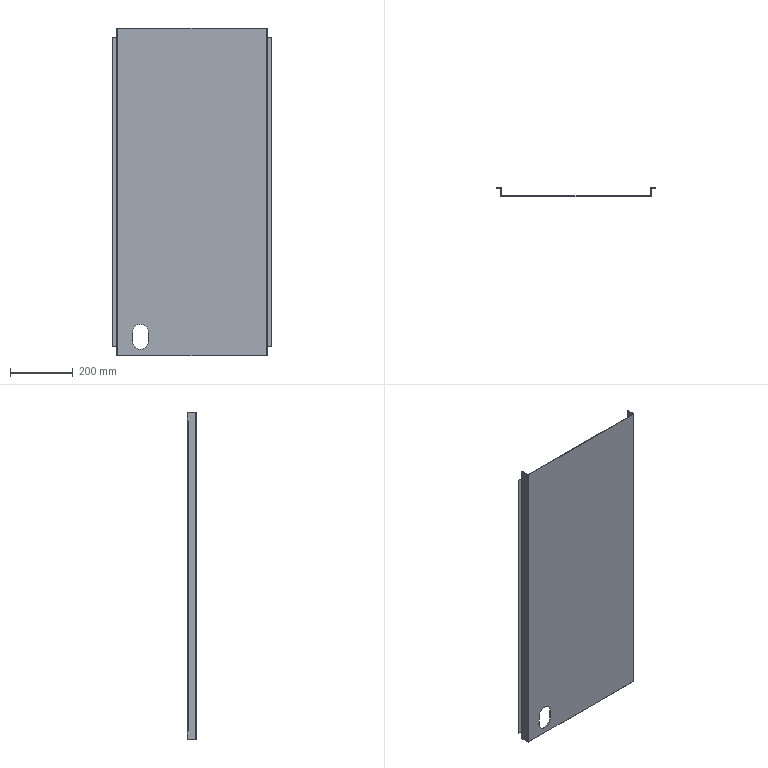Part | SolidWorks | features EdgeFlange 2, FlatPattern 1, ICE 1, SMBaseFlange 1, SheetMetal 1 | 1 solid | 51 faces | box 510 x 30 x 1047 mm | volume 876812 mm3 | plane 40 | cylinder 11 | commonest cylinder face diameters 3 x4 6 x4 50 x3
STEP:
#1=CARTESIAN_POINT('',(63.279,-16.571,45.));
#2=VERTEX_POINT('',#1);
#3=CARTESIAN_POINT('',(38.279,-16.571,20.));
#4=VERTEX_POINT('',#3);
#5=CARTESIAN_POINT('',(38.279,-16.571,45.));
#6=DIRECTION('',(0.,1.,0.));
#7=DIRECTION('',(0.,0.,1.));
#8=AXIS2_PLACEMENT_3D('',#5,#6,#7);
#9=CIRCLE('',#8,25.);
#10=EDGE_CURVE('',#2,#4,#9,.T.);
#11=ORIENTED_EDGE('',*,*,#10,.T.);
#12=CARTESIAN_POINT('',(38.279,-18.071,20.));
#13=VERTEX_POINT('',#12);
#14=CARTESIAN_POINT('',(38.279,-8.071,20.));
#15=DIRECTION('',(0.,-1.,0.));
#16=VECTOR('',#15,1000.);
#17=LINE('',#14,#16);
#18=EDGE_CURVE('',#4,#13,#17,.T.);
#19=ORIENTED_EDGE('',*,*,#18,.T.);
#20=CARTESIAN_POINT('',(63.279,-18.071,45.));
#21=VERTEX_POINT('',#20);
#22=CARTESIAN_POINT('',(38.279,-18.071,45.));
#23=DIRECTION('',(0.,-1.,0.));
#24=DIRECTION('',(0.,0.,-1.));
#25=AXIS2_PLACEMENT_3D('',#22,#23,#24);
#26=CIRCLE('',#25,25.);
#27=EDGE_CURVE('',#13,#21,#26,.T.);
#28=ORIENTED_EDGE('',*,*,#27,.T.);
#29=CARTESIAN_POINT('',(63.279,-8.071,45.));
#30=DIRECTION('',(0.,-1.,0.));
#31=VECTOR('',#30,1000.);
#32=LINE('',#29,#31);
#33=EDGE_CURVE('',#2,#21,#32,.T.);
#34=ORIENTED_EDGE('',*,*,#33,.F.);
#35=EDGE_LOOP('',(#11,#19,#28,#34));
#36=FACE_OUTER_BOUND('',#35,.T.);
#37=CARTESIAN_POINT('',(38.279,-8.071,45.));
#38=DIRECTION('',(0.,-1.,0.));
#39=DIRECTION('',(0.,0.,-1.));
#40=AXIS2_PLACEMENT_3D('',#37,#38,#39);
#41=CYLINDRICAL_SURFACE('',#40,25.);
#42=ADVANCED_FACE('',(#36),#41,.F.);
#43=CARTESIAN_POINT('',(-36.721,11.929,28.5));
#44=VERTEX_POINT('',#43);
#45=CARTESIAN_POINT('',(-36.721,11.527,28.5));
#46=VERTEX_POINT('',#45);
#47=CARTESIAN_POINT('',(-36.721,11.929,28.5));
#48=DIRECTION('',(0.,-1.,0.));
#49=VECTOR('',#48,1000.);
#50=LINE('',#47,#49);
#51=EDGE_CURVE('',#44,#46,#50,.T.);
#52=ORIENTED_EDGE('',*,*,#51,.T.);
#53=CARTESIAN_POINT('',(-35.221,8.929,28.5));
#54=VERTEX_POINT('',#53);
#55=CARTESIAN_POINT('',(-38.221,8.929,28.5));
#56=DIRECTION('',(0.,0.,-1.));
#57=DIRECTION('',(-1.,0.,0.));
#58=AXIS2_PLACEMENT_3D('',#55,#56,#57);
#59=CIRCLE('',#58,3.);
#60=EDGE_CURVE('',#46,#54,#59,.T.);
#61=ORIENTED_EDGE('',*,*,#60,.T.);
#62=CARTESIAN_POINT('',(-35.221,11.929,28.5));
#63=VERTEX_POINT('',#62);
#64=CARTESIAN_POINT('',(-35.221,0.,28.5));
#65=DIRECTION('',(0.,-1.,0.));
#66=VECTOR('',#65,1000.);
#67=LINE('',#64,#66);
#68=EDGE_CURVE('',#63,#54,#67,.T.);
#69=ORIENTED_EDGE('',*,*,#68,.F.);
#70=CARTESIAN_POINT('',(-36.721,11.929,28.5));
#71=DIRECTION('',(1.,0.,0.));
#72=VECTOR('',#71,1000.);
#73=LINE('',#70,#72);
#74=EDGE_CURVE('',#44,#63,#73,.T.);
#75=ORIENTED_EDGE('',*,*,#74,.F.);
#76=EDGE_LOOP('',(#52,#61,#69,#75));
#77=FACE_OUTER_BOUND('',#76,.T.);
#78=CARTESIAN_POINT('',(-36.721,11.929,28.5));
#79=DIRECTION('',(0.,0.,1.));
#80=DIRECTION('',(0.,-1.,0.));
#81=AXIS2_PLACEMENT_3D('',#78,#79,#80);
#82=PLANE('',#81);
#83=ADVANCED_FACE('',(#77),#82,.T.);
#84=CARTESIAN_POINT('',(-35.221,8.929,1018.5));
#85=VERTEX_POINT('',#84);
#86=CARTESIAN_POINT('',(-35.221,11.929,1018.5));
#87=VERTEX_POINT('',#86);
#88=CARTESIAN_POINT('',(-35.221,0.,1018.5));
#89=DIRECTION('',(0.,1.,0.));
#90=VECTOR('',#89,1000.);
#91=LINE('',#88,#90);
#92=EDGE_CURVE('',#85,#87,#91,.T.);
#93=ORIENTED_EDGE('',*,*,#92,.F.);
#94=CARTESIAN_POINT('',(-36.721,11.527,1018.5));
#95=VERTEX_POINT('',#94);
#96=CARTESIAN_POINT('',(-38.221,8.929,1018.5));
#97=DIRECTION('',(0.,0.,1.));
#98=DIRECTION('',(-1.,0.,0.));
#99=AXIS2_PLACEMENT_3D('',#96,#97,#98);
#100=CIRCLE('',#99,3.);
#101=EDGE_CURVE('',#85,#95,#100,.T.);
#102=ORIENTED_EDGE('',*,*,#101,.T.);
#103=CARTESIAN_POINT('',(-36.721,11.929,1018.5));
#104=VERTEX_POINT('',#103);
#105=CARTESIAN_POINT('',(-36.721,8.929,1018.5));
#106=DIRECTION('',(0.,1.,0.));
#107=VECTOR('',#106,1000.);
#108=LINE('',#105,#107);
#109=EDGE_CURVE('',#95,#104,#108,.T.);
#110=ORIENTED_EDGE('',*,*,#109,.T.);
#111=CARTESIAN_POINT('',(-36.721,11.929,1018.5));
#112=DIRECTION('',(1.,0.,0.));
#113=VECTOR('',#112,1000.);
#114=LINE('',#111,#113);
#115=EDGE_CURVE('',#104,#87,#114,.T.);
#116=ORIENTED_EDGE('',*,*,#115,.T.);
#117=EDGE_LOOP('',(#93,#102,#110,#116));
#118=FACE_OUTER_BOUND('',#117,.T.);
#119=CARTESIAN_POINT('',(-36.721,8.929,1018.5));
#120=DIRECTION('',(0.,0.,-1.));
#121=DIRECTION('',(-1.,0.,0.));
#122=AXIS2_PLACEMENT_3D('',#119,#120,#121);
#123=PLANE('',#122);
#124=ADVANCED_FACE('',(#118),#123,.T.);
#125=CARTESIAN_POINT('',(443.279,11.929,1018.5));
#126=VERTEX_POINT('',#125);
#127=CARTESIAN_POINT('',(443.279,11.527,1018.5));
#128=VERTEX_POINT('',#127);
#129=CARTESIAN_POINT('',(443.279,11.929,1018.5));
#130=DIRECTION('',(0.,-1.,0.));
#131=VECTOR('',#130,1000.);
#132=LINE('',#129,#131);
#133=EDGE_CURVE('',#126,#128,#132,.T.);
#134=ORIENTED_EDGE('',*,*,#133,.T.);
#135=CARTESIAN_POINT('',(441.779,8.929,1018.5));
#136=VERTEX_POINT('',#135);
#137=CARTESIAN_POINT('',(444.779,8.929,1018.5));
#138=DIRECTION('',(0.,0.,1.));
#139=DIRECTION('',(1.,0.,0.));
#140=AXIS2_PLACEMENT_3D('',#137,#138,#139);
#141=CIRCLE('',#140,3.);
#142=EDGE_CURVE('',#128,#136,#141,.T.);
#143=ORIENTED_EDGE('',*,*,#142,.T.);
#144=CARTESIAN_POINT('',(441.779,11.929,1018.5));
#145=VERTEX_POINT('',#144);
#146=CARTESIAN_POINT('',(441.779,0.,1018.5));
#147=DIRECTION('',(0.,1.,0.));
#148=VECTOR('',#147,1000.);
#149=LINE('',#146,#148);
#150=EDGE_CURVE('',#136,#145,#149,.T.);
#151=ORIENTED_EDGE('',*,*,#150,.T.);
#152=CARTESIAN_POINT('',(443.279,11.929,1018.5));
#153=DIRECTION('',(-1.,0.,0.));
#154=VECTOR('',#153,1000.);
#155=LINE('',#152,#154);
#156=EDGE_CURVE('',#126,#145,#155,.T.);
#157=ORIENTED_EDGE('',*,*,#156,.F.);
#158=EDGE_LOOP('',(#134,#143,#151,#157));
#159=FACE_OUTER_BOUND('',#158,.T.);
#160=CARTESIAN_POINT('',(443.279,11.929,1018.5));
#161=DIRECTION('',(0.,0.,-1.));
#162=DIRECTION('',(-1.,0.,0.));
#163=AXIS2_PLACEMENT_3D('',#160,#161,#162);
#164=PLANE('',#163);
#165=ADVANCED_FACE('',(#159),#164,.T.);
#166=CARTESIAN_POINT('',(441.779,11.929,28.5));
#167=VERTEX_POINT('',#166);
#168=CARTESIAN_POINT('',(441.779,8.929,28.5));
#169=VERTEX_POINT('',#168);
#170=CARTESIAN_POINT('',(441.779,0.,28.5));
#171=DIRECTION('',(0.,-1.,0.));
#172=VECTOR('',#171,1000.);
#173=LINE('',#170,#172);
#174=EDGE_CURVE('',#167,#169,#173,.T.);
#175=ORIENTED_EDGE('',*,*,#174,.T.);
#176=CARTESIAN_POINT('',(443.279,11.527,28.5));
#177=VERTEX_POINT('',#176);
#178=CARTESIAN_POINT('',(444.779,8.929,28.5));
#179=DIRECTION('',(0.,0.,-1.));
#180=DIRECTION('',(1.,0.,0.));
#181=AXIS2_PLACEMENT_3D('',#178,#179,#180);
#182=CIRCLE('',#181,3.);
#183=EDGE_CURVE('',#169,#177,#182,.T.);
#184=ORIENTED_EDGE('',*,*,#183,.T.);
#185=CARTESIAN_POINT('',(443.279,11.929,28.5));
#186=VERTEX_POINT('',#185);
#187=CARTESIAN_POINT('',(443.279,8.929,28.5));
#188=DIRECTION('',(0.,1.,0.));
#189=VECTOR('',#188,1000.);
#190=LINE('',#187,#189);
#191=EDGE_CURVE('',#177,#186,#190,.T.);
#192=ORIENTED_EDGE('',*,*,#191,.T.);
#193=CARTESIAN_POINT('',(443.279,11.929,28.5));
#194=DIRECTION('',(-1.,0.,0.));
#195=VECTOR('',#194,1000.);
#196=LINE('',#193,#195);
#197=EDGE_CURVE('',#186,#167,#196,.T.);
#198=ORIENTED_EDGE('',*,*,#197,.T.);
#199=EDGE_LOOP('',(#175,#184,#192,#198));
#200=FACE_OUTER_BOUND('',#199,.T.);
#201=CARTESIAN_POINT('',(443.279,8.929,28.5));
#202=DIRECTION('',(0.,0.,1.));
#203=DIRECTION('',(1.,0.,0.));
#204=AXIS2_PLACEMENT_3D('',#201,#202,#203);
#205=PLANE('',#204);
#206=ADVANCED_FACE('',(#200),#205,.T.);
#207=ORIENTED_EDGE('',*,*,#51,.F.);
#208=CARTESIAN_POINT('',(-36.721,11.929,0.));
#209=VERTEX_POINT('',#208);
#210=CARTESIAN_POINT('',(-36.721,11.929,0.));
#211=DIRECTION('',(0.,0.,1.));
#212=VECTOR('',#211,1000.);
#213=LINE('',#210,#212);
#214=EDGE_CURVE('',#209,#44,#213,.T.);
#215=ORIENTED_EDGE('',*,*,#214,.F.);
#216=CARTESIAN_POINT('',(-36.721,-15.071,0.));
#217=VERTEX_POINT('',#216);
#218=CARTESIAN_POINT('',(-36.721,-16.571,0.));
#219=DIRECTION('',(0.,1.,0.));
#220=VECTOR('',#219,1000.);
#221=LINE('',#218,#220);
#222=EDGE_CURVE('',#217,#209,#221,.T.);
#223=ORIENTED_EDGE('',*,*,#222,.F.);
#224=CARTESIAN_POINT('',(-36.721,-15.071,1047.));
#225=VERTEX_POINT('',#224);
#226=CARTESIAN_POINT('',(-36.721,-15.071,0.));
#227=DIRECTION('',(0.,0.,-1.));
#228=VECTOR('',#227,1000.);
#229=LINE('',#226,#228);
#230=EDGE_CURVE('',#225,#217,#229,.T.);
#231=ORIENTED_EDGE('',*,*,#230,.F.);
#232=CARTESIAN_POINT('',(-36.721,11.929,1047.));
#233=VERTEX_POINT('',#232);
#234=CARTESIAN_POINT('',(-36.721,11.929,1047.));
#235=DIRECTION('',(0.,-1.,0.));
#236=VECTOR('',#235,1000.);
#237=LINE('',#234,#236);
#238=EDGE_CURVE('',#233,#225,#237,.T.);
#239=ORIENTED_EDGE('',*,*,#238,.F.);
#240=CARTESIAN_POINT('',(-36.721,11.929,0.));
#241=DIRECTION('',(0.,0.,1.));
#242=VECTOR('',#241,1000.);
#243=LINE('',#240,#242);
#244=EDGE_CURVE('',#104,#233,#243,.T.);
#245=ORIENTED_EDGE('',*,*,#244,.F.);
#246=ORIENTED_EDGE('',*,*,#109,.F.);
#247=CARTESIAN_POINT('',(-36.721,8.929,1018.5));
#248=VERTEX_POINT('',#247);
#249=CARTESIAN_POINT('',(-36.721,8.929,1018.5));
#250=DIRECTION('',(0.,1.,0.));
#251=VECTOR('',#250,1000.);
#252=LINE('',#249,#251);
#253=EDGE_CURVE('',#248,#95,#252,.T.);
#254=ORIENTED_EDGE('',*,*,#253,.F.);
#255=CARTESIAN_POINT('',(-36.721,8.929,28.5));
#256=VERTEX_POINT('',#255);
#257=CARTESIAN_POINT('',(-36.721,8.929,28.5));
#258=DIRECTION('',(0.,0.,1.));
#259=VECTOR('',#258,1000.);
#260=LINE('',#257,#259);
#261=EDGE_CURVE('',#256,#248,#260,.T.);
#262=ORIENTED_EDGE('',*,*,#261,.F.);
#263=CARTESIAN_POINT('',(-36.721,11.929,28.5));
#264=DIRECTION('',(0.,-1.,0.));
#265=VECTOR('',#264,1000.);
#266=LINE('',#263,#265);
#267=EDGE_CURVE('',#46,#256,#266,.T.);
#268=ORIENTED_EDGE('',*,*,#267,.F.);
#269=EDGE_LOOP('',(#207,#215,#223,#231,#239,#245,#246,#254,#262,#268));
#270=FACE_OUTER_BOUND('',#269,.T.);
#271=CARTESIAN_POINT('',(-36.721,0.,0.));
#272=DIRECTION('',(1.,0.,0.));
#273=DIRECTION('',(0.,1.,0.));
#274=AXIS2_PLACEMENT_3D('',#271,#272,#273);
#275=PLANE('',#274);
#276=ADVANCED_FACE('',(#270),#275,.F.);
#277=CARTESIAN_POINT('',(-35.221,11.929,0.));
#278=VERTEX_POINT('',#277);
#279=CARTESIAN_POINT('',(-35.221,11.929,0.));
#280=DIRECTION('',(0.,0.,1.));
#281=VECTOR('',#280,1000.);
#282=LINE('',#279,#281);
#283=EDGE_CURVE('',#278,#63,#282,.T.);
#284=ORIENTED_EDGE('',*,*,#283,.T.);
#285=ORIENTED_EDGE('',*,*,#68,.T.);
#286=CARTESIAN_POINT('',(-35.221,8.929,28.5));
#287=DIRECTION('',(0.,0.,1.));
#288=VECTOR('',#287,1000.);
#289=LINE('',#286,#288);
#290=EDGE_CURVE('',#54,#85,#289,.T.);
#291=ORIENTED_EDGE('',*,*,#290,.T.);
#292=ORIENTED_EDGE('',*,*,#92,.T.);
#293=CARTESIAN_POINT('',(-35.221,11.929,1047.));
#294=VERTEX_POINT('',#293);
#295=CARTESIAN_POINT('',(-35.221,11.929,0.));
#296=DIRECTION('',(0.,0.,1.));
#297=VECTOR('',#296,1000.);
#298=LINE('',#295,#297);
#299=EDGE_CURVE('',#87,#294,#298,.T.);
#300=ORIENTED_EDGE('',*,*,#299,.T.);
#301=CARTESIAN_POINT('',(-35.221,-15.071,1047.));
#302=VERTEX_POINT('',#301);
#303=CARTESIAN_POINT('',(-35.221,0.,1047.));
#304=DIRECTION('',(0.,-1.,0.));
#305=VECTOR('',#304,1000.);
#306=LINE('',#303,#305);
#307=EDGE_CURVE('',#294,#302,#306,.T.);
#308=ORIENTED_EDGE('',*,*,#307,.T.);
#309=CARTESIAN_POINT('',(-35.221,-15.071,0.));
#310=VERTEX_POINT('',#309);
#311=CARTESIAN_POINT('',(-35.221,-15.071,0.));
#312=DIRECTION('',(0.,0.,1.));
#313=VECTOR('',#312,1000.);
#314=LINE('',#311,#313);
#315=EDGE_CURVE('',#310,#302,#314,.T.);
#316=ORIENTED_EDGE('',*,*,#315,.F.);
#317=CARTESIAN_POINT('',(-35.221,0.,0.));
#318=DIRECTION('',(0.,1.,0.));
#319=VECTOR('',#318,1000.);
#320=LINE('',#317,#319);
#321=EDGE_CURVE('',#310,#278,#320,.T.);
#322=ORIENTED_EDGE('',*,*,#321,.T.);
#323=EDGE_LOOP('',(#284,#285,#291,#292,#300,#308,#316,#322));
#324=FACE_OUTER_BOUND('',#323,.T.);
#325=CARTESIAN_POINT('',(-35.221,0.,0.));
#326=DIRECTION('',(1.,0.,0.));
#327=DIRECTION('',(0.,1.,0.));
#328=AXIS2_PLACEMENT_3D('',#325,#326,#327);
#329=PLANE('',#328);
#330=ADVANCED_FACE('',(#324),#329,.T.);
#331=ORIENTED_EDGE('',*,*,#214,.T.);
#332=ORIENTED_EDGE('',*,*,#74,.T.);
#333=ORIENTED_EDGE('',*,*,#283,.F.);
#334=CARTESIAN_POINT('',(-36.721,11.929,0.));
#335=DIRECTION('',(1.,0.,0.));
#336=VECTOR('',#335,1000.);
#337=LINE('',#334,#336);
#338=EDGE_CURVE('',#209,#278,#337,.T.);
#339=ORIENTED_EDGE('',*,*,#338,.F.);
#340=EDGE_LOOP('',(#331,#332,#333,#339));
#341=FACE_OUTER_BOUND('',#340,.T.);
#342=CARTESIAN_POINT('',(-36.721,11.929,0.));
#343=DIRECTION('',(0.,1.,0.));
#344=DIRECTION('',(-1.,0.,0.));
#345=AXIS2_PLACEMENT_3D('',#342,#343,#344);
#346=PLANE('',#345);
#347=ADVANCED_FACE('',(#341),#346,.T.);
#348=ORIENTED_EDGE('',*,*,#299,.F.);
#349=ORIENTED_EDGE('',*,*,#115,.F.);
#350=ORIENTED_EDGE('',*,*,#244,.T.);
#351=CARTESIAN_POINT('',(-36.721,11.929,1047.));
#352=DIRECTION('',(1.,0.,0.));
#353=VECTOR('',#352,1000.);
#354=LINE('',#351,#353);
#355=EDGE_CURVE('',#233,#294,#354,.T.);
#356=ORIENTED_EDGE('',*,*,#355,.T.);
#357=EDGE_LOOP('',(#348,#349,#350,#356));
#358=FACE_OUTER_BOUND('',#357,.T.);
#359=CARTESIAN_POINT('',(-36.721,11.929,0.));
#360=DIRECTION('',(0.,1.,0.));
#361=DIRECTION('',(-1.,0.,0.));
#362=AXIS2_PLACEMENT_3D('',#359,#360,#361);
#363=PLANE('',#362);
#364=ADVANCED_FACE('',(#358),#363,.T.);
#365=CARTESIAN_POINT('',(443.279,8.929,1018.5));
#366=VERTEX_POINT('',#365);
#367=CARTESIAN_POINT('',(443.279,8.929,28.5));
#368=VERTEX_POINT('',#367);
#369=CARTESIAN_POINT('',(443.279,8.929,1018.5));
#370=DIRECTION('',(0.,0.,-1.));
#371=VECTOR('',#370,1000.);
#372=LINE('',#369,#371);
#373=EDGE_CURVE('',#366,#368,#372,.T.);
#374=ORIENTED_EDGE('',*,*,#373,.F.);
#375=CARTESIAN_POINT('',(443.279,11.929,1018.5));
#376=DIRECTION('',(0.,-1.,0.));
#377=VECTOR('',#376,1000.);
#378=LINE('',#375,#377);
#379=EDGE_CURVE('',#128,#366,#378,.T.);
#380=ORIENTED_EDGE('',*,*,#379,.F.);
#381=ORIENTED_EDGE('',*,*,#133,.F.);
#382=CARTESIAN_POINT('',(443.279,11.929,1047.));
#383=VERTEX_POINT('',#382);
#384=CARTESIAN_POINT('',(443.279,11.929,0.));
#385=DIRECTION('',(0.,0.,-1.));
#386=VECTOR('',#385,1000.);
#387=LINE('',#384,#386);
#388=EDGE_CURVE('',#383,#126,#387,.T.);
#389=ORIENTED_EDGE('',*,*,#388,.F.);
#390=CARTESIAN_POINT('',(443.279,-15.071,1047.));
#391=VERTEX_POINT('',#390);
#392=CARTESIAN_POINT('',(443.279,11.929,1047.));
#393=DIRECTION('',(0.,1.,0.));
#394=VECTOR('',#393,1000.);
#395=LINE('',#392,#394);
#396=EDGE_CURVE('',#391,#383,#395,.T.);
#397=ORIENTED_EDGE('',*,*,#396,.F.);
#398=CARTESIAN_POINT('',(443.279,-15.071,0.));
#399=VERTEX_POINT('',#398);
#400=CARTESIAN_POINT('',(443.279,-15.071,0.));
#401=DIRECTION('',(0.,0.,-1.));
#402=VECTOR('',#401,1000.);
#403=LINE('',#400,#402);
#404=EDGE_CURVE('',#391,#399,#403,.T.);
#405=ORIENTED_EDGE('',*,*,#404,.T.);
#406=CARTESIAN_POINT('',(443.279,11.929,0.));
#407=VERTEX_POINT('',#406);
#408=CARTESIAN_POINT('',(443.279,-16.571,0.));
#409=DIRECTION('',(0.,-1.,0.));
#410=VECTOR('',#409,1000.);
#411=LINE('',#408,#410);
#412=EDGE_CURVE('',#407,#399,#411,.T.);
#413=ORIENTED_EDGE('',*,*,#412,.F.);
#414=CARTESIAN_POINT('',(443.279,11.929,0.));
#415=DIRECTION('',(0.,0.,-1.));
#416=VECTOR('',#415,1000.);
#417=LINE('',#414,#416);
#418=EDGE_CURVE('',#186,#407,#417,.T.);
#419=ORIENTED_EDGE('',*,*,#418,.F.);
#420=ORIENTED_EDGE('',*,*,#191,.F.);
#421=CARTESIAN_POINT('',(443.279,8.929,28.5));
#422=DIRECTION('',(0.,1.,0.));
#423=VECTOR('',#422,1000.);
#424=LINE('',#421,#423);
#425=EDGE_CURVE('',#368,#177,#424,.T.);
#426=ORIENTED_EDGE('',*,*,#425,.F.);
#427=EDGE_LOOP('',(#374,#380,#381,#389,#397,#405,#413,#419,#420,#426));
#428=FACE_OUTER_BOUND('',#427,.T.);
#429=CARTESIAN_POINT('',(443.279,0.,0.));
#430=DIRECTION('',(1.,0.,0.));
#431=DIRECTION('',(0.,1.,0.));
#432=AXIS2_PLACEMENT_3D('',#429,#430,#431);
#433=PLANE('',#432);
#434=ADVANCED_FACE('',(#428),#433,.T.);
#435=ORIENTED_EDGE('',*,*,#150,.F.);
#436=CARTESIAN_POINT('',(441.779,8.929,1018.5));
#437=DIRECTION('',(0.,0.,-1.));
#438=VECTOR('',#437,1000.);
#439=LINE('',#436,#438);
#440=EDGE_CURVE('',#136,#169,#439,.T.);
#441=ORIENTED_EDGE('',*,*,#440,.T.);
#442=ORIENTED_EDGE('',*,*,#174,.F.);
#443=CARTESIAN_POINT('',(441.779,11.929,0.));
#444=VERTEX_POINT('',#443);
#445=CARTESIAN_POINT('',(441.779,11.929,0.));
#446=DIRECTION('',(0.,0.,-1.));
#447=VECTOR('',#446,1000.);
#448=LINE('',#445,#447);
#449=EDGE_CURVE('',#167,#444,#448,.T.);
#450=ORIENTED_EDGE('',*,*,#449,.T.);
#451=CARTESIAN_POINT('',(441.779,-15.071,0.));
#452=VERTEX_POINT('',#451);
#453=CARTESIAN_POINT('',(441.779,0.,0.));
#454=DIRECTION('',(0.,-1.,0.));
#455=VECTOR('',#454,1000.);
#456=LINE('',#453,#455);
#457=EDGE_CURVE('',#444,#452,#456,.T.);
#458=ORIENTED_EDGE('',*,*,#457,.T.);
#459=CARTESIAN_POINT('',(441.779,-15.071,1047.));
#460=VERTEX_POINT('',#459);
#461=CARTESIAN_POINT('',(441.779,-15.071,1047.));
#462=DIRECTION('',(0.,0.,-1.));
#463=VECTOR('',#462,1000.);
#464=LINE('',#461,#463);
#465=EDGE_CURVE('',#460,#452,#464,.T.);
#466=ORIENTED_EDGE('',*,*,#465,.F.);
#467=CARTESIAN_POINT('',(441.779,11.929,1047.));
#468=VERTEX_POINT('',#467);
#469=CARTESIAN_POINT('',(441.779,0.,1047.));
#470=DIRECTION('',(0.,1.,0.));
#471=VECTOR('',#470,1000.);
#472=LINE('',#469,#471);
#473=EDGE_CURVE('',#460,#468,#472,.T.);
#474=ORIENTED_EDGE('',*,*,#473,.T.);
#475=CARTESIAN_POINT('',(441.779,11.929,0.));
#476=DIRECTION('',(0.,0.,-1.));
#477=VECTOR('',#476,1000.);
#478=LINE('',#475,#477);
#479=EDGE_CURVE('',#468,#145,#478,.T.);
#480=ORIENTED_EDGE('',*,*,#479,.T.);
#481=EDGE_LOOP('',(#435,#441,#442,#450,#458,#466,#474,#480));
#482=FACE_OUTER_BOUND('',#481,.T.);
#483=CARTESIAN_POINT('',(441.779,0.,0.));
#484=DIRECTION('',(1.,0.,0.));
#485=DIRECTION('',(0.,1.,0.));
#486=AXIS2_PLACEMENT_3D('',#483,#484,#485);
#487=PLANE('',#486);
#488=ADVANCED_FACE('',(#482),#487,.F.);
#489=ORIENTED_EDGE('',*,*,#388,.T.);
#490=ORIENTED_EDGE('',*,*,#156,.T.);
#491=ORIENTED_EDGE('',*,*,#479,.F.);
#492=CARTESIAN_POINT('',(443.279,11.929,1047.));
#493=DIRECTION('',(-1.,0.,0.));
#494=VECTOR('',#493,1000.);
#495=LINE('',#492,#494);
#496=EDGE_CURVE('',#383,#468,#495,.T.);
#497=ORIENTED_EDGE('',*,*,#496,.F.);
#498=EDGE_LOOP('',(#489,#490,#491,#497));
#499=FACE_OUTER_BOUND('',#498,.T.);
#500=CARTESIAN_POINT('',(443.279,11.929,0.));
#501=DIRECTION('',(0.,1.,0.));
#502=DIRECTION('',(-1.,0.,0.));
#503=AXIS2_PLACEMENT_3D('',#500,#501,#502);
#504=PLANE('',#503);
#505=ADVANCED_FACE('',(#499),#504,.T.);
#506=ORIENTED_EDGE('',*,*,#449,.F.);
#507=ORIENTED_EDGE('',*,*,#197,.F.);
#508=ORIENTED_EDGE('',*,*,#418,.T.);
#509=CARTESIAN_POINT('',(443.279,11.929,0.));
#510=DIRECTION('',(-1.,0.,0.));
#511=VECTOR('',#510,1000.);
#512=LINE('',#509,#511);
#513=EDGE_CURVE('',#407,#444,#512,.T.);
#514=ORIENTED_EDGE('',*,*,#513,.T.);
#515=EDGE_LOOP('',(#506,#507,#508,#514));
#516=FACE_OUTER_BOUND('',#515,.T.);
#517=CARTESIAN_POINT('',(443.279,11.929,0.));
#518=DIRECTION('',(0.,1.,0.));
#519=DIRECTION('',(-1.,0.,0.));
#520=AXIS2_PLACEMENT_3D('',#517,#518,#519);
#521=PLANE('',#520);
#522=ADVANCED_FACE('',(#516),#521,.T.);
#523=CARTESIAN_POINT('',(13.279,-18.071,75.));
#524=VERTEX_POINT('',#523);
#525=CARTESIAN_POINT('',(13.279,-18.071,45.));
#526=VERTEX_POINT('',#525);
#527=CARTESIAN_POINT('',(13.279,-18.071,75.));
#528=DIRECTION('',(0.,0.,-1.));
#529=VECTOR('',#528,1000.);
#530=LINE('',#527,#529);
#531=EDGE_CURVE('',#524,#526,#530,.T.);
#532=ORIENTED_EDGE('',*,*,#531,.F.);
#533=CARTESIAN_POINT('',(63.279,-18.071,75.));
#534=VERTEX_POINT('',#533);
#535=CARTESIAN_POINT('',(38.279,-18.071,75.));
#536=DIRECTION('',(0.,-1.,0.));
#537=DIRECTION('',(0.,0.,-1.));
#538=AXIS2_PLACEMENT_3D('',#535,#536,#537);
#539=CIRCLE('',#538,25.);
#540=EDGE_CURVE('',#534,#524,#539,.T.);
#541=ORIENTED_EDGE('',*,*,#540,.F.);
#542=CARTESIAN_POINT('',(63.279,-18.071,75.));
#543=DIRECTION('',(0.,0.,1.));
#544=VECTOR('',#543,1000.);
#545=LINE('',#542,#544);
#546=EDGE_CURVE('',#21,#534,#545,.T.);
#547=ORIENTED_EDGE('',*,*,#546,.F.);
#548=ORIENTED_EDGE('',*,*,#27,.F.);
#549=CARTESIAN_POINT('',(38.279,-18.071,45.));
#550=DIRECTION('',(0.,-1.,0.));
#551=DIRECTION('',(0.,0.,-1.));
#552=AXIS2_PLACEMENT_3D('',#549,#550,#551);
#553=CIRCLE('',#552,25.);
#554=EDGE_CURVE('',#526,#13,#553,.T.);
#555=ORIENTED_EDGE('',*,*,#554,.F.);
#556=EDGE_LOOP('',(#532,#541,#547,#548,#555));
#557=FACE_BOUND('',#556,.T.);
#558=CARTESIAN_POINT('',(-33.721,-18.071,1047.));
#559=VERTEX_POINT('',#558);
#560=CARTESIAN_POINT('',(-33.721,-18.071,0.));
#561=VERTEX_POINT('',#560);
#562=CARTESIAN_POINT('',(-33.721,-18.071,1047.));
#563=DIRECTION('',(0.,0.,-1.));
#564=VECTOR('',#563,1000.);
#565=LINE('',#562,#564);
#566=EDGE_CURVE('',#559,#561,#565,.T.);
#567=ORIENTED_EDGE('',*,*,#566,.T.);
#568=CARTESIAN_POINT('',(440.279,-18.071,0.));
#569=VERTEX_POINT('',#568);
#570=CARTESIAN_POINT('',(-36.721,-18.071,0.));
#571=DIRECTION('',(1.,0.,0.));
#572=VECTOR('',#571,1000.);
#573=LINE('',#570,#572);
#574=EDGE_CURVE('',#561,#569,#573,.T.);
#575=ORIENTED_EDGE('',*,*,#574,.T.);
#576=CARTESIAN_POINT('',(440.279,-18.071,1047.));
#577=VERTEX_POINT('',#576);
#578=CARTESIAN_POINT('',(440.279,-18.071,0.));
#579=DIRECTION('',(0.,0.,1.));
#580=VECTOR('',#579,1000.);
#581=LINE('',#578,#580);
#582=EDGE_CURVE('',#569,#577,#581,.T.);
#583=ORIENTED_EDGE('',*,*,#582,.T.);
#584=CARTESIAN_POINT('',(-36.721,-18.071,1047.));
#585=DIRECTION('',(1.,0.,0.));
#586=VECTOR('',#585,1000.);
#587=LINE('',#584,#586);
#588=EDGE_CURVE('',#559,#577,#587,.T.);
#589=ORIENTED_EDGE('',*,*,#588,.F.);
#590=EDGE_LOOP('',(#567,#575,#583,#589));
#591=FACE_OUTER_BOUND('',#590,.T.);
#592=CARTESIAN_POINT('',(-36.721,-18.071,1047.));
#593=DIRECTION('',(0.,1.,0.));
#594=DIRECTION('',(0.,0.,1.));
#595=AXIS2_PLACEMENT_3D('',#592,#593,#594);
#596=PLANE('',#595);
#597=ADVANCED_FACE('',(#557,#591),#596,.F.);
#598=CARTESIAN_POINT('',(13.279,-16.571,75.));
#599=VERTEX_POINT('',#598);
#600=CARTESIAN_POINT('',(63.279,-16.571,75.));
#601=VERTEX_POINT('',#600);
#602=CARTESIAN_POINT('',(38.279,-16.571,75.));
#603=DIRECTION('',(0.,1.,0.));
#604=DIRECTION('',(0.,0.,1.));
#605=AXIS2_PLACEMENT_3D('',#602,#603,#604);
#606=CIRCLE('',#605,25.);
#607=EDGE_CURVE('',#599,#601,#606,.T.);
#608=ORIENTED_EDGE('',*,*,#607,.F.);
#609=CARTESIAN_POINT('',(13.279,-16.571,45.));
#610=VERTEX_POINT('',#609);
#611=CARTESIAN_POINT('',(13.279,-16.571,1047.));
#612=DIRECTION('',(0.,0.,1.));
#613=VECTOR('',#612,1000.);
#614=LINE('',#611,#613);
#615=EDGE_CURVE('',#610,#599,#614,.T.);
#616=ORIENTED_EDGE('',*,*,#615,.F.);
#617=CARTESIAN_POINT('',(38.279,-16.571,45.));
#618=DIRECTION('',(0.,1.,0.));
#619=DIRECTION('',(0.,0.,1.));
#620=AXIS2_PLACEMENT_3D('',#617,#618,#619);
#621=CIRCLE('',#620,25.);
#622=EDGE_CURVE('',#4,#610,#621,.T.);
#623=ORIENTED_EDGE('',*,*,#622,.F.);
#624=ORIENTED_EDGE('',*,*,#10,.F.);
#625=CARTESIAN_POINT('',(63.279,-16.571,1047.));
#626=DIRECTION('',(0.,0.,-1.));
#627=VECTOR('',#626,1000.);
#628=LINE('',#625,#627);
#629=EDGE_CURVE('',#601,#2,#628,.T.);
#630=ORIENTED_EDGE('',*,*,#629,.F.);
#631=EDGE_LOOP('',(#608,#616,#623,#624,#630));
#632=FACE_BOUND('',#631,.T.);
#633=CARTESIAN_POINT('',(-33.721,-16.571,0.));
#634=VERTEX_POINT('',#633);
#635=CARTESIAN_POINT('',(440.279,-16.571,0.));
#636=VERTEX_POINT('',#635);
#637=CARTESIAN_POINT('',(-36.721,-16.571,0.));
#638=DIRECTION('',(1.,0.,0.));
#639=VECTOR('',#638,1000.);
#640=LINE('',#637,#639);
#641=EDGE_CURVE('',#634,#636,#640,.T.);
#642=ORIENTED_EDGE('',*,*,#641,.F.);
#643=CARTESIAN_POINT('',(-33.721,-16.571,1047.));
#644=VERTEX_POINT('',#643);
#645=CARTESIAN_POINT('',(-33.721,-16.571,1047.));
#646=DIRECTION('',(0.,0.,-1.));
#647=VECTOR('',#646,1000.);
#648=LINE('',#645,#647);
#649=EDGE_CURVE('',#644,#634,#648,.T.);
#650=ORIENTED_EDGE('',*,*,#649,.F.);
#651=CARTESIAN_POINT('',(440.279,-16.571,1047.));
#652=VERTEX_POINT('',#651);
#653=CARTESIAN_POINT('',(-36.721,-16.571,1047.));
#654=DIRECTION('',(1.,0.,0.));
#655=VECTOR('',#654,1000.);
#656=LINE('',#653,#655);
#657=EDGE_CURVE('',#644,#652,#656,.T.);
#658=ORIENTED_EDGE('',*,*,#657,.T.);
#659=CARTESIAN_POINT('',(440.279,-16.571,0.));
#660=DIRECTION('',(0.,0.,1.));
#661=VECTOR('',#660,1000.);
#662=LINE('',#659,#661);
#663=EDGE_CURVE('',#636,#652,#662,.T.);
#664=ORIENTED_EDGE('',*,*,#663,.F.);
#665=EDGE_LOOP('',(#642,#650,#658,#664));
#666=FACE_OUTER_BOUND('',#665,.T.);
#667=CARTESIAN_POINT('',(-36.721,-16.571,1047.));
#668=DIRECTION('',(0.,1.,0.));
#669=DIRECTION('',(0.,0.,1.));
#670=AXIS2_PLACEMENT_3D('',#667,#668,#669);
#671=PLANE('',#670);
#672=ADVANCED_FACE('',(#632,#666),#671,.T.);
#673=CARTESIAN_POINT('',(-33.721,-16.571,1047.));
#674=DIRECTION('',(0.,-1.,0.));
#675=VECTOR('',#674,1000.);
#676=LINE('',#673,#675);
#677=EDGE_CURVE('',#644,#559,#676,.T.);
#678=ORIENTED_EDGE('',*,*,#677,.T.);
#679=ORIENTED_EDGE('',*,*,#588,.T.);
#680=CARTESIAN_POINT('',(440.279,-16.571,1047.));
#681=DIRECTION('',(0.,-1.,0.));
#682=VECTOR('',#681,1000.);
#683=LINE('',#680,#682);
#684=EDGE_CURVE('',#652,#577,#683,.T.);
#685=ORIENTED_EDGE('',*,*,#684,.F.);
#686=ORIENTED_EDGE('',*,*,#657,.F.);
#687=EDGE_LOOP('',(#678,#679,#685,#686));
#688=FACE_OUTER_BOUND('',#687,.T.);
#689=CARTESIAN_POINT('',(0.,0.,1047.));
#690=DIRECTION('',(0.,0.,-1.));
#691=DIRECTION('',(-1.,0.,0.));
#692=AXIS2_PLACEMENT_3D('',#689,#690,#691);
#693=PLANE('',#692);
#694=ADVANCED_FACE('',(#688),#693,.F.);
#695=CARTESIAN_POINT('',(-33.721,-16.571,0.));
#696=DIRECTION('',(0.,-1.,0.));
#697=VECTOR('',#696,1000.);
#698=LINE('',#695,#697);
#699=EDGE_CURVE('',#634,#561,#698,.T.);
#700=ORIENTED_EDGE('',*,*,#699,.F.);
#701=ORIENTED_EDGE('',*,*,#641,.T.);
#702=CARTESIAN_POINT('',(440.279,-16.571,0.));
#703=DIRECTION('',(0.,-1.,0.));
#704=VECTOR('',#703,1000.);
#705=LINE('',#702,#704);
#706=EDGE_CURVE('',#636,#569,#705,.T.);
#707=ORIENTED_EDGE('',*,*,#706,.T.);
#708=ORIENTED_EDGE('',*,*,#574,.F.);
#709=EDGE_LOOP('',(#700,#701,#707,#708));
#710=FACE_OUTER_BOUND('',#709,.T.);
#711=CARTESIAN_POINT('',(0.,0.,0.));
#712=DIRECTION('',(0.,0.,-1.));
#713=DIRECTION('',(-1.,0.,0.));
#714=AXIS2_PLACEMENT_3D('',#711,#712,#713);
#715=PLANE('',#714);
#716=ADVANCED_FACE('',(#710),#715,.T.);
#717=CARTESIAN_POINT('',(443.279,-15.071,1047.));
#718=DIRECTION('',(1.,0.,0.));
#719=VECTOR('',#718,1000.);
#720=LINE('',#717,#719);
#721=EDGE_CURVE('',#460,#391,#720,.T.);
#722=ORIENTED_EDGE('',*,*,#721,.F.);
#723=CARTESIAN_POINT('',(440.279,-15.071,1047.));
#724=DIRECTION('',(0.,0.,1.));
#725=DIRECTION('',(0.,1.,0.));
#726=AXIS2_PLACEMENT_3D('',#723,#724,#725);
#727=CIRCLE('',#726,1.5);
#728=EDGE_CURVE('',#652,#460,#727,.T.);
#729=ORIENTED_EDGE('',*,*,#728,.F.);
#730=ORIENTED_EDGE('',*,*,#684,.T.);
#731=CARTESIAN_POINT('',(440.279,-15.071,1047.));
#732=DIRECTION('',(0.,0.,1.));
#733=DIRECTION('',(0.,1.,0.));
#734=AXIS2_PLACEMENT_3D('',#731,#732,#733);
#735=CIRCLE('',#734,3.);
#736=EDGE_CURVE('',#577,#391,#735,.T.);
#737=ORIENTED_EDGE('',*,*,#736,.T.);
#738=EDGE_LOOP('',(#722,#729,#730,#737));
#739=FACE_OUTER_BOUND('',#738,.T.);
#740=CARTESIAN_POINT('',(440.279,-15.071,1047.));
#741=DIRECTION('',(0.,0.,1.));
#742=DIRECTION('',(0.,-1.,0.));
#743=AXIS2_PLACEMENT_3D('',#740,#741,#742);
#744=PLANE('',#743);
#745=ADVANCED_FACE('',(#739),#744,.T.);
#746=CARTESIAN_POINT('',(440.279,-15.071,0.));
#747=DIRECTION('',(0.,0.,-1.));
#748=DIRECTION('',(0.,1.,0.));
#749=AXIS2_PLACEMENT_3D('',#746,#747,#748);
#750=CIRCLE('',#749,1.5);
#751=EDGE_CURVE('',#452,#636,#750,.T.);
#752=ORIENTED_EDGE('',*,*,#751,.F.);
#753=CARTESIAN_POINT('',(441.779,-15.071,0.));
#754=DIRECTION('',(1.,0.,0.));
#755=VECTOR('',#754,1000.);
#756=LINE('',#753,#755);
#757=EDGE_CURVE('',#452,#399,#756,.T.);
#758=ORIENTED_EDGE('',*,*,#757,.T.);
#759=CARTESIAN_POINT('',(440.279,-15.071,0.));
#760=DIRECTION('',(0.,0.,-1.));
#761=DIRECTION('',(0.,1.,0.));
#762=AXIS2_PLACEMENT_3D('',#759,#760,#761);
#763=CIRCLE('',#762,3.);
#764=EDGE_CURVE('',#399,#569,#763,.T.);
#765=ORIENTED_EDGE('',*,*,#764,.T.);
#766=ORIENTED_EDGE('',*,*,#706,.F.);
#767=EDGE_LOOP('',(#752,#758,#765,#766));
#768=FACE_OUTER_BOUND('',#767,.T.);
#769=CARTESIAN_POINT('',(440.279,-15.071,0.));
#770=DIRECTION('',(0.,0.,1.));
#771=DIRECTION('',(0.,-1.,0.));
#772=AXIS2_PLACEMENT_3D('',#769,#770,#771);
#773=PLANE('',#772);
#774=ADVANCED_FACE('',(#768),#773,.F.);
#775=ORIENTED_EDGE('',*,*,#582,.F.);
#776=ORIENTED_EDGE('',*,*,#764,.F.);
#777=ORIENTED_EDGE('',*,*,#404,.F.);
#778=ORIENTED_EDGE('',*,*,#736,.F.);
#779=EDGE_LOOP('',(#775,#776,#777,#778));
#780=FACE_OUTER_BOUND('',#779,.T.);
#781=CARTESIAN_POINT('',(440.279,-15.071,0.));
#782=DIRECTION('',(0.,0.,-1.));
#783=DIRECTION('',(1.,0.,0.));
#784=AXIS2_PLACEMENT_3D('',#781,#782,#783);
#785=CYLINDRICAL_SURFACE('',#784,3.);
#786=ADVANCED_FACE('',(#780),#785,.T.);
#787=ORIENTED_EDGE('',*,*,#663,.T.);
#788=ORIENTED_EDGE('',*,*,#728,.T.);
#789=ORIENTED_EDGE('',*,*,#465,.T.);
#790=ORIENTED_EDGE('',*,*,#751,.T.);
#791=EDGE_LOOP('',(#787,#788,#789,#790));
#792=FACE_OUTER_BOUND('',#791,.T.);
#793=CARTESIAN_POINT('',(440.279,-15.071,0.));
#794=DIRECTION('',(0.,0.,-1.));
#795=DIRECTION('',(1.,0.,0.));
#796=AXIS2_PLACEMENT_3D('',#793,#794,#795);
#797=CYLINDRICAL_SURFACE('',#796,1.5);
#798=ADVANCED_FACE('',(#792),#797,.F.);
#799=ORIENTED_EDGE('',*,*,#412,.T.);
#800=ORIENTED_EDGE('',*,*,#757,.F.);
#801=ORIENTED_EDGE('',*,*,#457,.F.);
#802=ORIENTED_EDGE('',*,*,#513,.F.);
#803=EDGE_LOOP('',(#799,#800,#801,#802));
#804=FACE_OUTER_BOUND('',#803,.T.);
#805=CARTESIAN_POINT('',(443.279,-16.571,0.));
#806=DIRECTION('',(0.,0.,-1.));
#807=DIRECTION('',(-1.,0.,0.));
#808=AXIS2_PLACEMENT_3D('',#805,#806,#807);
#809=PLANE('',#808);
#810=ADVANCED_FACE('',(#804),#809,.T.);
#811=ORIENTED_EDGE('',*,*,#473,.F.);
#812=ORIENTED_EDGE('',*,*,#721,.T.);
#813=ORIENTED_EDGE('',*,*,#396,.T.);
#814=ORIENTED_EDGE('',*,*,#496,.T.);
#815=EDGE_LOOP('',(#811,#812,#813,#814));
#816=FACE_OUTER_BOUND('',#815,.T.);
#817=CARTESIAN_POINT('',(443.279,11.929,1047.));
#818=DIRECTION('',(0.,0.,1.));
#819=DIRECTION('',(1.,0.,0.));
#820=AXIS2_PLACEMENT_3D('',#817,#818,#819);
#821=PLANE('',#820);
#822=ADVANCED_FACE('',(#816),#821,.T.);
#823=CARTESIAN_POINT('',(-36.721,-15.071,0.));
#824=DIRECTION('',(-1.,0.,0.));
#825=VECTOR('',#824,1000.);
#826=LINE('',#823,#825);
#827=EDGE_CURVE('',#310,#217,#826,.T.);
#828=ORIENTED_EDGE('',*,*,#827,.F.);
#829=CARTESIAN_POINT('',(-33.721,-15.071,0.));
#830=DIRECTION('',(0.,0.,-1.));
#831=DIRECTION('',(1.,0.,0.));
#832=AXIS2_PLACEMENT_3D('',#829,#830,#831);
#833=CIRCLE('',#832,1.5);
#834=EDGE_CURVE('',#634,#310,#833,.T.);
#835=ORIENTED_EDGE('',*,*,#834,.F.);
#836=ORIENTED_EDGE('',*,*,#699,.T.);
#837=CARTESIAN_POINT('',(-33.721,-15.071,0.));
#838=DIRECTION('',(0.,0.,-1.));
#839=DIRECTION('',(1.,0.,0.));
#840=AXIS2_PLACEMENT_3D('',#837,#838,#839);
#841=CIRCLE('',#840,3.);
#842=EDGE_CURVE('',#561,#217,#841,.T.);
#843=ORIENTED_EDGE('',*,*,#842,.T.);
#844=EDGE_LOOP('',(#828,#835,#836,#843));
#845=FACE_OUTER_BOUND('',#844,.T.);
#846=CARTESIAN_POINT('',(-33.721,-15.071,0.));
#847=DIRECTION('',(0.,0.,-1.));
#848=DIRECTION('',(-1.,0.,0.));
#849=AXIS2_PLACEMENT_3D('',#846,#847,#848);
#850=PLANE('',#849);
#851=ADVANCED_FACE('',(#845),#850,.T.);
#852=CARTESIAN_POINT('',(-33.721,-15.071,1047.));
#853=DIRECTION('',(0.,0.,1.));
#854=DIRECTION('',(1.,0.,0.));
#855=AXIS2_PLACEMENT_3D('',#852,#853,#854);
#856=CIRCLE('',#855,1.5);
#857=EDGE_CURVE('',#302,#644,#856,.T.);
#858=ORIENTED_EDGE('',*,*,#857,.F.);
#859=CARTESIAN_POINT('',(-35.221,-15.071,1047.));
#860=DIRECTION('',(-1.,0.,0.));
#861=VECTOR('',#860,1000.);
#862=LINE('',#859,#861);
#863=EDGE_CURVE('',#302,#225,#862,.T.);
#864=ORIENTED_EDGE('',*,*,#863,.T.);
#865=CARTESIAN_POINT('',(-33.721,-15.071,1047.));
#866=DIRECTION('',(0.,0.,1.));
#867=DIRECTION('',(1.,0.,0.));
#868=AXIS2_PLACEMENT_3D('',#865,#866,#867);
#869=CIRCLE('',#868,3.);
#870=EDGE_CURVE('',#225,#559,#869,.T.);
#871=ORIENTED_EDGE('',*,*,#870,.T.);
#872=ORIENTED_EDGE('',*,*,#677,.F.);
#873=EDGE_LOOP('',(#858,#864,#871,#872));
#874=FACE_OUTER_BOUND('',#873,.T.);
#875=CARTESIAN_POINT('',(-33.721,-15.071,1047.));
#876=DIRECTION('',(0.,0.,-1.));
#877=DIRECTION('',(-1.,0.,0.));
#878=AXIS2_PLACEMENT_3D('',#875,#876,#877);
#879=PLANE('',#878);
#880=ADVANCED_FACE('',(#874),#879,.F.);
#881=ORIENTED_EDGE('',*,*,#566,.F.);
#882=ORIENTED_EDGE('',*,*,#870,.F.);
#883=ORIENTED_EDGE('',*,*,#230,.T.);
#884=ORIENTED_EDGE('',*,*,#842,.F.);
#885=EDGE_LOOP('',(#881,#882,#883,#884));
#886=FACE_OUTER_BOUND('',#885,.T.);
#887=CARTESIAN_POINT('',(-33.721,-15.071,1047.));
#888=DIRECTION('',(0.,0.,1.));
#889=DIRECTION('',(-1.,0.,0.));
#890=AXIS2_PLACEMENT_3D('',#887,#888,#889);
#891=CYLINDRICAL_SURFACE('',#890,3.);
#892=ADVANCED_FACE('',(#886),#891,.T.);
#893=ORIENTED_EDGE('',*,*,#649,.T.);
#894=ORIENTED_EDGE('',*,*,#834,.T.);
#895=ORIENTED_EDGE('',*,*,#315,.T.);
#896=ORIENTED_EDGE('',*,*,#857,.T.);
#897=EDGE_LOOP('',(#893,#894,#895,#896));
#898=FACE_OUTER_BOUND('',#897,.T.);
#899=CARTESIAN_POINT('',(-33.721,-15.071,1047.));
#900=DIRECTION('',(0.,0.,1.));
#901=DIRECTION('',(-1.,0.,0.));
#902=AXIS2_PLACEMENT_3D('',#899,#900,#901);
#903=CYLINDRICAL_SURFACE('',#902,1.5);
#904=ADVANCED_FACE('',(#898),#903,.F.);
#905=ORIENTED_EDGE('',*,*,#321,.F.);
#906=ORIENTED_EDGE('',*,*,#827,.T.);
#907=ORIENTED_EDGE('',*,*,#222,.T.);
#908=ORIENTED_EDGE('',*,*,#338,.T.);
#909=EDGE_LOOP('',(#905,#906,#907,#908));
#910=FACE_OUTER_BOUND('',#909,.T.);
#911=CARTESIAN_POINT('',(-36.721,-16.571,0.));
#912=DIRECTION('',(0.,0.,-1.));
#913=DIRECTION('',(-1.,0.,0.));
#914=AXIS2_PLACEMENT_3D('',#911,#912,#913);
#915=PLANE('',#914);
#916=ADVANCED_FACE('',(#910),#915,.T.);
#917=ORIENTED_EDGE('',*,*,#238,.T.);
#918=ORIENTED_EDGE('',*,*,#863,.F.);
#919=ORIENTED_EDGE('',*,*,#307,.F.);
#920=ORIENTED_EDGE('',*,*,#355,.F.);
#921=EDGE_LOOP('',(#917,#918,#919,#920));
#922=FACE_OUTER_BOUND('',#921,.T.);
#923=CARTESIAN_POINT('',(-36.721,11.929,1047.));
#924=DIRECTION('',(0.,0.,1.));
#925=DIRECTION('',(1.,0.,0.));
#926=AXIS2_PLACEMENT_3D('',#923,#924,#925);
#927=PLANE('',#926);
#928=ADVANCED_FACE('',(#922),#927,.T.);
#929=CARTESIAN_POINT('',(444.779,10.429,28.5));
#930=VERTEX_POINT('',#929);
#931=CARTESIAN_POINT('',(444.779,8.929,28.5));
#932=DIRECTION('',(0.,0.,-1.));
#933=DIRECTION('',(1.,0.,0.));
#934=AXIS2_PLACEMENT_3D('',#931,#932,#933);
#935=CIRCLE('',#934,1.5);
#936=EDGE_CURVE('',#368,#930,#935,.T.);
#937=ORIENTED_EDGE('',*,*,#936,.F.);
#938=ORIENTED_EDGE('',*,*,#425,.T.);
#939=CARTESIAN_POINT('',(444.779,11.929,28.5));
#940=VERTEX_POINT('',#939);
#941=CARTESIAN_POINT('',(444.779,8.929,28.5));
#942=DIRECTION('',(0.,0.,-1.));
#943=DIRECTION('',(1.,0.,0.));
#944=AXIS2_PLACEMENT_3D('',#941,#942,#943);
#945=CIRCLE('',#944,3.);
#946=EDGE_CURVE('',#177,#940,#945,.T.);
#947=ORIENTED_EDGE('',*,*,#946,.T.);
#948=CARTESIAN_POINT('',(444.779,11.929,28.5));
#949=DIRECTION('',(0.,1.,0.));
#950=VECTOR('',#949,1000.);
#951=LINE('',#948,#950);
#952=EDGE_CURVE('',#930,#940,#951,.T.);
#953=ORIENTED_EDGE('',*,*,#952,.F.);
#954=EDGE_LOOP('',(#937,#938,#947,#953));
#955=FACE_OUTER_BOUND('',#954,.T.);
#956=CARTESIAN_POINT('',(444.779,8.929,28.5));
#957=DIRECTION('',(0.,0.,-1.));
#958=DIRECTION('',(-1.,0.,0.));
#959=AXIS2_PLACEMENT_3D('',#956,#957,#958);
#960=PLANE('',#959);
#961=ADVANCED_FACE('',(#955),#960,.T.);
#962=CARTESIAN_POINT('',(444.779,11.929,1018.5));
#963=VERTEX_POINT('',#962);
#964=CARTESIAN_POINT('',(444.779,8.929,1018.5));
#965=DIRECTION('',(0.,0.,1.));
#966=DIRECTION('',(1.,0.,0.));
#967=AXIS2_PLACEMENT_3D('',#964,#965,#966);
#968=CIRCLE('',#967,3.);
#969=EDGE_CURVE('',#963,#128,#968,.T.);
#970=ORIENTED_EDGE('',*,*,#969,.T.);
#971=ORIENTED_EDGE('',*,*,#379,.T.);
#972=CARTESIAN_POINT('',(444.779,10.429,1018.5));
#973=VERTEX_POINT('',#972);
#974=CARTESIAN_POINT('',(444.779,8.929,1018.5));
#975=DIRECTION('',(0.,0.,1.));
#976=DIRECTION('',(1.,0.,0.));
#977=AXIS2_PLACEMENT_3D('',#974,#975,#976);
#978=CIRCLE('',#977,1.5);
#979=EDGE_CURVE('',#973,#366,#978,.T.);
#980=ORIENTED_EDGE('',*,*,#979,.F.);
#981=CARTESIAN_POINT('',(444.779,10.429,1018.5));
#982=DIRECTION('',(0.,1.,0.));
#983=VECTOR('',#982,1000.);
#984=LINE('',#981,#983);
#985=EDGE_CURVE('',#973,#963,#984,.T.);
#986=ORIENTED_EDGE('',*,*,#985,.T.);
#987=EDGE_LOOP('',(#970,#971,#980,#986));
#988=FACE_OUTER_BOUND('',#987,.T.);
#989=CARTESIAN_POINT('',(444.779,8.929,1018.5));
#990=DIRECTION('',(0.,0.,-1.));
#991=DIRECTION('',(-1.,0.,0.));
#992=AXIS2_PLACEMENT_3D('',#989,#990,#991);
#993=PLANE('',#992);
#994=ADVANCED_FACE('',(#988),#993,.F.);
#995=ORIENTED_EDGE('',*,*,#440,.F.);
#996=ORIENTED_EDGE('',*,*,#142,.F.);
#997=ORIENTED_EDGE('',*,*,#969,.F.);
#998=CARTESIAN_POINT('',(444.779,11.929,28.5));
#999=DIRECTION('',(0.,0.,-1.));
#1000=VECTOR('',#999,1000.);
#1001=LINE('',#998,#1000);
#1002=EDGE_CURVE('',#963,#940,#1001,.T.);
#1003=ORIENTED_EDGE('',*,*,#1002,.T.);
#1004=ORIENTED_EDGE('',*,*,#946,.F.);
#1005=ORIENTED_EDGE('',*,*,#183,.F.);
#1006=EDGE_LOOP('',(#995,#996,#997,#1003,#1004,#1005));
#1007=FACE_OUTER_BOUND('',#1006,.T.);
#1008=CARTESIAN_POINT('',(444.779,8.929,1018.5));
#1009=DIRECTION('',(0.,0.,1.));
#1010=DIRECTION('',(0.,1.,0.));
#1011=AXIS2_PLACEMENT_3D('',#1008,#1009,#1010);
#1012=CYLINDRICAL_SURFACE('',#1011,3.);
#1013=ADVANCED_FACE('',(#1007),#1012,.T.);
#1014=ORIENTED_EDGE('',*,*,#373,.T.);
#1015=ORIENTED_EDGE('',*,*,#936,.T.);
#1016=CARTESIAN_POINT('',(444.779,10.429,28.5));
#1017=DIRECTION('',(0.,0.,1.));
#1018=VECTOR('',#1017,1000.);
#1019=LINE('',#1016,#1018);
#1020=EDGE_CURVE('',#930,#973,#1019,.T.);
#1021=ORIENTED_EDGE('',*,*,#1020,.T.);
#1022=ORIENTED_EDGE('',*,*,#979,.T.);
#1023=EDGE_LOOP('',(#1014,#1015,#1021,#1022));
#1024=FACE_OUTER_BOUND('',#1023,.T.);
#1025=CARTESIAN_POINT('',(444.779,8.929,1018.5));
#1026=DIRECTION('',(0.,0.,1.));
#1027=DIRECTION('',(0.,1.,0.));
#1028=AXIS2_PLACEMENT_3D('',#1025,#1026,#1027);
#1029=CYLINDRICAL_SURFACE('',#1028,1.5);
#1030=ADVANCED_FACE('',(#1024),#1029,.F.);
#1031=ORIENTED_EDGE('',*,*,#985,.F.);
#1032=CARTESIAN_POINT('',(458.279,10.429,1018.5));
#1033=VERTEX_POINT('',#1032);
#1034=CARTESIAN_POINT('',(458.279,10.429,1018.5));
#1035=DIRECTION('',(1.,0.,0.));
#1036=VECTOR('',#1035,1000.);
#1037=LINE('',#1034,#1036);
#1038=EDGE_CURVE('',#973,#1033,#1037,.T.);
#1039=ORIENTED_EDGE('',*,*,#1038,.T.);
#1040=CARTESIAN_POINT('',(458.279,11.929,1018.5));
#1041=VERTEX_POINT('',#1040);
#1042=CARTESIAN_POINT('',(458.279,11.929,1018.5));
#1043=DIRECTION('',(0.,-1.,0.));
#1044=VECTOR('',#1043,1000.);
#1045=LINE('',#1042,#1044);
#1046=EDGE_CURVE('',#1041,#1033,#1045,.T.);
#1047=ORIENTED_EDGE('',*,*,#1046,.F.);
#1048=CARTESIAN_POINT('',(0.,11.929,1018.5));
#1049=DIRECTION('',(1.,0.,0.));
#1050=VECTOR('',#1049,1000.);
#1051=LINE('',#1048,#1050);
#1052=EDGE_CURVE('',#963,#1041,#1051,.T.);
#1053=ORIENTED_EDGE('',*,*,#1052,.F.);
#1054=EDGE_LOOP('',(#1031,#1039,#1047,#1053));
#1055=FACE_OUTER_BOUND('',#1054,.T.);
#1056=CARTESIAN_POINT('',(458.279,11.929,1018.5));
#1057=DIRECTION('',(0.,0.,-1.));
#1058=DIRECTION('',(0.,1.,0.));
#1059=AXIS2_PLACEMENT_3D('',#1056,#1057,#1058);
#1060=PLANE('',#1059);
#1061=ADVANCED_FACE('',(#1055),#1060,.F.);
#1062=ORIENTED_EDGE('',*,*,#952,.T.);
#1063=CARTESIAN_POINT('',(458.279,11.929,28.5));
#1064=VERTEX_POINT('',#1063);
#1065=CARTESIAN_POINT('',(0.,11.929,28.5));
#1066=DIRECTION('',(-1.,0.,0.));
#1067=VECTOR('',#1066,1000.);
#1068=LINE('',#1065,#1067);
#1069=EDGE_CURVE('',#1064,#940,#1068,.T.);
#1070=ORIENTED_EDGE('',*,*,#1069,.F.);
#1071=CARTESIAN_POINT('',(458.279,10.429,28.5));
#1072=VERTEX_POINT('',#1071);
#1073=CARTESIAN_POINT('',(458.279,11.929,28.5));
#1074=DIRECTION('',(0.,-1.,0.));
#1075=VECTOR('',#1074,1000.);
#1076=LINE('',#1073,#1075);
#1077=EDGE_CURVE('',#1064,#1072,#1076,.T.);
#1078=ORIENTED_EDGE('',*,*,#1077,.T.);
#1079=CARTESIAN_POINT('',(443.279,10.429,28.5));
#1080=DIRECTION('',(-1.,0.,0.));
#1081=VECTOR('',#1080,1000.);
#1082=LINE('',#1079,#1081);
#1083=EDGE_CURVE('',#1072,#930,#1082,.T.);
#1084=ORIENTED_EDGE('',*,*,#1083,.T.);
#1085=EDGE_LOOP('',(#1062,#1070,#1078,#1084));
#1086=FACE_OUTER_BOUND('',#1085,.T.);
#1087=CARTESIAN_POINT('',(443.279,11.929,28.5));
#1088=DIRECTION('',(0.,0.,1.));
#1089=DIRECTION('',(1.,0.,0.));
#1090=AXIS2_PLACEMENT_3D('',#1087,#1088,#1089);
#1091=PLANE('',#1090);
#1092=ADVANCED_FACE('',(#1086),#1091,.F.);
#1093=ORIENTED_EDGE('',*,*,#1002,.F.);
#1094=ORIENTED_EDGE('',*,*,#1052,.T.);
#1095=CARTESIAN_POINT('',(458.279,11.929,0.));
#1096=DIRECTION('',(0.,0.,-1.));
#1097=VECTOR('',#1096,1000.);
#1098=LINE('',#1095,#1097);
#1099=EDGE_CURVE('',#1041,#1064,#1098,.T.);
#1100=ORIENTED_EDGE('',*,*,#1099,.T.);
#1101=ORIENTED_EDGE('',*,*,#1069,.T.);
#1102=EDGE_LOOP('',(#1093,#1094,#1100,#1101));
#1103=FACE_OUTER_BOUND('',#1102,.T.);
#1104=CARTESIAN_POINT('',(0.,11.929,0.));
#1105=DIRECTION('',(0.,-1.,0.));
#1106=DIRECTION('',(1.,0.,0.));
#1107=AXIS2_PLACEMENT_3D('',#1104,#1105,#1106);
#1108=PLANE('',#1107);
#1109=ADVANCED_FACE('',(#1103),#1108,.F.);
#1110=ORIENTED_EDGE('',*,*,#1038,.F.);
#1111=ORIENTED_EDGE('',*,*,#1020,.F.);
#1112=ORIENTED_EDGE('',*,*,#1083,.F.);
#1113=CARTESIAN_POINT('',(458.279,10.429,28.5));
#1114=DIRECTION('',(0.,0.,-1.));
#1115=VECTOR('',#1114,1000.);
#1116=LINE('',#1113,#1115);
#1117=EDGE_CURVE('',#1033,#1072,#1116,.T.);
#1118=ORIENTED_EDGE('',*,*,#1117,.F.);
#1119=EDGE_LOOP('',(#1110,#1111,#1112,#1118));
#1120=FACE_OUTER_BOUND('',#1119,.T.);
#1121=CARTESIAN_POINT('',(0.,10.429,0.));
#1122=DIRECTION('',(0.,-1.,0.));
#1123=DIRECTION('',(1.,0.,0.));
#1124=AXIS2_PLACEMENT_3D('',#1121,#1122,#1123);
#1125=PLANE('',#1124);
#1126=ADVANCED_FACE('',(#1120),#1125,.T.);
#1127=ORIENTED_EDGE('',*,*,#1117,.T.);
#1128=ORIENTED_EDGE('',*,*,#1077,.F.);
#1129=ORIENTED_EDGE('',*,*,#1099,.F.);
#1130=ORIENTED_EDGE('',*,*,#1046,.T.);
#1131=EDGE_LOOP('',(#1127,#1128,#1129,#1130));
#1132=FACE_OUTER_BOUND('',#1131,.T.);
#1133=CARTESIAN_POINT('',(458.279,11.929,28.5));
#1134=DIRECTION('',(-1.,0.,0.));
#1135=DIRECTION('',(0.,-1.,0.));
#1136=AXIS2_PLACEMENT_3D('',#1133,#1134,#1135);
#1137=PLANE('',#1136);
#1138=ADVANCED_FACE('',(#1132),#1137,.F.);
#1139=CARTESIAN_POINT('',(-38.221,10.429,1018.5));
#1140=VERTEX_POINT('',#1139);
#1141=CARTESIAN_POINT('',(-38.221,8.929,1018.5));
#1142=DIRECTION('',(0.,0.,1.));
#1143=DIRECTION('',(-1.,0.,0.));
#1144=AXIS2_PLACEMENT_3D('',#1141,#1142,#1143);
#1145=CIRCLE('',#1144,1.5);
#1146=EDGE_CURVE('',#248,#1140,#1145,.T.);
#1147=ORIENTED_EDGE('',*,*,#1146,.F.);
#1148=ORIENTED_EDGE('',*,*,#253,.T.);
#1149=CARTESIAN_POINT('',(-38.221,11.929,1018.5));
#1150=VERTEX_POINT('',#1149);
#1151=CARTESIAN_POINT('',(-38.221,8.929,1018.5));
#1152=DIRECTION('',(0.,0.,1.));
#1153=DIRECTION('',(-1.,0.,0.));
#1154=AXIS2_PLACEMENT_3D('',#1151,#1152,#1153);
#1155=CIRCLE('',#1154,3.);
#1156=EDGE_CURVE('',#95,#1150,#1155,.T.);
#1157=ORIENTED_EDGE('',*,*,#1156,.T.);
#1158=CARTESIAN_POINT('',(-38.221,11.929,1018.5));
#1159=DIRECTION('',(0.,1.,0.));
#1160=VECTOR('',#1159,1000.);
#1161=LINE('',#1158,#1160);
#1162=EDGE_CURVE('',#1140,#1150,#1161,.T.);
#1163=ORIENTED_EDGE('',*,*,#1162,.F.);
#1164=EDGE_LOOP('',(#1147,#1148,#1157,#1163));
#1165=FACE_OUTER_BOUND('',#1164,.T.);
#1166=CARTESIAN_POINT('',(-38.221,8.929,1018.5));
#1167=DIRECTION('',(0.,0.,1.));
#1168=DIRECTION('',(1.,0.,0.));
#1169=AXIS2_PLACEMENT_3D('',#1166,#1167,#1168);
#1170=PLANE('',#1169);
#1171=ADVANCED_FACE('',(#1165),#1170,.T.);
#1172=CARTESIAN_POINT('',(-38.221,11.929,28.5));
#1173=VERTEX_POINT('',#1172);
#1174=CARTESIAN_POINT('',(-38.221,8.929,28.5));
#1175=DIRECTION('',(0.,0.,-1.));
#1176=DIRECTION('',(-1.,0.,0.));
#1177=AXIS2_PLACEMENT_3D('',#1174,#1175,#1176);
#1178=CIRCLE('',#1177,3.);
#1179=EDGE_CURVE('',#1173,#46,#1178,.T.);
#1180=ORIENTED_EDGE('',*,*,#1179,.T.);
#1181=ORIENTED_EDGE('',*,*,#267,.T.);
#1182=CARTESIAN_POINT('',(-38.221,10.429,28.5));
#1183=VERTEX_POINT('',#1182);
#1184=CARTESIAN_POINT('',(-38.221,8.929,28.5));
#1185=DIRECTION('',(0.,0.,-1.));
#1186=DIRECTION('',(-1.,0.,0.));
#1187=AXIS2_PLACEMENT_3D('',#1184,#1185,#1186);
#1188=CIRCLE('',#1187,1.5);
#1189=EDGE_CURVE('',#1183,#256,#1188,.T.);
#1190=ORIENTED_EDGE('',*,*,#1189,.F.);
#1191=CARTESIAN_POINT('',(-38.221,10.429,28.5));
#1192=DIRECTION('',(0.,1.,0.));
#1193=VECTOR('',#1192,1000.);
#1194=LINE('',#1191,#1193);
#1195=EDGE_CURVE('',#1183,#1173,#1194,.T.);
#1196=ORIENTED_EDGE('',*,*,#1195,.T.);
#1197=EDGE_LOOP('',(#1180,#1181,#1190,#1196));
#1198=FACE_OUTER_BOUND('',#1197,.T.);
#1199=CARTESIAN_POINT('',(-38.221,8.929,28.5));
#1200=DIRECTION('',(0.,0.,1.));
#1201=DIRECTION('',(1.,0.,0.));
#1202=AXIS2_PLACEMENT_3D('',#1199,#1200,#1201);
#1203=PLANE('',#1202);
#1204=ADVANCED_FACE('',(#1198),#1203,.F.);
#1205=ORIENTED_EDGE('',*,*,#290,.F.);
#1206=ORIENTED_EDGE('',*,*,#60,.F.);
#1207=ORIENTED_EDGE('',*,*,#1179,.F.);
#1208=CARTESIAN_POINT('',(-38.221,11.929,1018.5));
#1209=DIRECTION('',(0.,0.,1.));
#1210=VECTOR('',#1209,1000.);
#1211=LINE('',#1208,#1210);
#1212=EDGE_CURVE('',#1173,#1150,#1211,.T.);
#1213=ORIENTED_EDGE('',*,*,#1212,.T.);
#1214=ORIENTED_EDGE('',*,*,#1156,.F.);
#1215=ORIENTED_EDGE('',*,*,#101,.F.);
#1216=EDGE_LOOP('',(#1205,#1206,#1207,#1213,#1214,#1215));
#1217=FACE_OUTER_BOUND('',#1216,.T.);
#1218=CARTESIAN_POINT('',(-38.221,8.929,28.5));
#1219=DIRECTION('',(0.,0.,-1.));
#1220=DIRECTION('',(0.,1.,0.));
#1221=AXIS2_PLACEMENT_3D('',#1218,#1219,#1220);
#1222=CYLINDRICAL_SURFACE('',#1221,3.);
#1223=ADVANCED_FACE('',(#1217),#1222,.T.);
#1224=ORIENTED_EDGE('',*,*,#261,.T.);
#1225=ORIENTED_EDGE('',*,*,#1146,.T.);
#1226=CARTESIAN_POINT('',(-38.221,10.429,1018.5));
#1227=DIRECTION('',(0.,0.,-1.));
#1228=VECTOR('',#1227,1000.);
#1229=LINE('',#1226,#1228);
#1230=EDGE_CURVE('',#1140,#1183,#1229,.T.);
#1231=ORIENTED_EDGE('',*,*,#1230,.T.);
#1232=ORIENTED_EDGE('',*,*,#1189,.T.);
#1233=EDGE_LOOP('',(#1224,#1225,#1231,#1232));
#1234=FACE_OUTER_BOUND('',#1233,.T.);
#1235=CARTESIAN_POINT('',(-38.221,8.929,28.5));
#1236=DIRECTION('',(0.,0.,-1.));
#1237=DIRECTION('',(0.,1.,0.));
#1238=AXIS2_PLACEMENT_3D('',#1235,#1236,#1237);
#1239=CYLINDRICAL_SURFACE('',#1238,1.5);
#1240=ADVANCED_FACE('',(#1234),#1239,.F.);
#1241=ORIENTED_EDGE('',*,*,#1195,.F.);
#1242=CARTESIAN_POINT('',(-51.721,10.429,28.5));
#1243=VERTEX_POINT('',#1242);
#1244=CARTESIAN_POINT('',(-51.721,10.429,28.5));
#1245=DIRECTION('',(-1.,0.,0.));
#1246=VECTOR('',#1245,1000.);
#1247=LINE('',#1244,#1246);
#1248=EDGE_CURVE('',#1183,#1243,#1247,.T.);
#1249=ORIENTED_EDGE('',*,*,#1248,.T.);
#1250=CARTESIAN_POINT('',(-51.721,11.929,28.5));
#1251=VERTEX_POINT('',#1250);
#1252=CARTESIAN_POINT('',(-51.721,11.929,28.5));
#1253=DIRECTION('',(0.,-1.,0.));
#1254=VECTOR('',#1253,1000.);
#1255=LINE('',#1252,#1254);
#1256=EDGE_CURVE('',#1251,#1243,#1255,.T.);
#1257=ORIENTED_EDGE('',*,*,#1256,.F.);
#1258=CARTESIAN_POINT('',(0.,11.929,28.5));
#1259=DIRECTION('',(-1.,0.,0.));
#1260=VECTOR('',#1259,1000.);
#1261=LINE('',#1258,#1260);
#1262=EDGE_CURVE('',#1173,#1251,#1261,.T.);
#1263=ORIENTED_EDGE('',*,*,#1262,.F.);
#1264=EDGE_LOOP('',(#1241,#1249,#1257,#1263));
#1265=FACE_OUTER_BOUND('',#1264,.T.);
#1266=CARTESIAN_POINT('',(-51.721,11.929,28.5));
#1267=DIRECTION('',(0.,0.,1.));
#1268=DIRECTION('',(1.,0.,0.));
#1269=AXIS2_PLACEMENT_3D('',#1266,#1267,#1268);
#1270=PLANE('',#1269);
#1271=ADVANCED_FACE('',(#1265),#1270,.F.);
#1272=ORIENTED_EDGE('',*,*,#1162,.T.);
#1273=CARTESIAN_POINT('',(-51.721,11.929,1018.5));
#1274=VERTEX_POINT('',#1273);
#1275=CARTESIAN_POINT('',(0.,11.929,1018.5));
#1276=DIRECTION('',(1.,0.,0.));
#1277=VECTOR('',#1276,1000.);
#1278=LINE('',#1275,#1277);
#1279=EDGE_CURVE('',#1274,#1150,#1278,.T.);
#1280=ORIENTED_EDGE('',*,*,#1279,.F.);
#1281=CARTESIAN_POINT('',(-51.721,10.429,1018.5));
#1282=VERTEX_POINT('',#1281);
#1283=CARTESIAN_POINT('',(-51.721,11.929,1018.5));
#1284=DIRECTION('',(0.,-1.,0.));
#1285=VECTOR('',#1284,1000.);
#1286=LINE('',#1283,#1285);
#1287=EDGE_CURVE('',#1274,#1282,#1286,.T.);
#1288=ORIENTED_EDGE('',*,*,#1287,.T.);
#1289=CARTESIAN_POINT('',(-36.721,10.429,1018.5));
#1290=DIRECTION('',(1.,0.,0.));
#1291=VECTOR('',#1290,1000.);
#1292=LINE('',#1289,#1291);
#1293=EDGE_CURVE('',#1282,#1140,#1292,.T.);
#1294=ORIENTED_EDGE('',*,*,#1293,.T.);
#1295=EDGE_LOOP('',(#1272,#1280,#1288,#1294));
#1296=FACE_OUTER_BOUND('',#1295,.T.);
#1297=CARTESIAN_POINT('',(-36.721,11.929,1018.5));
#1298=DIRECTION('',(0.,0.,-1.));
#1299=DIRECTION('',(0.,1.,0.));
#1300=AXIS2_PLACEMENT_3D('',#1297,#1298,#1299);
#1301=PLANE('',#1300);
#1302=ADVANCED_FACE('',(#1296),#1301,.F.);
#1303=ORIENTED_EDGE('',*,*,#1212,.F.);
#1304=ORIENTED_EDGE('',*,*,#1262,.T.);
#1305=CARTESIAN_POINT('',(-51.721,11.929,0.));
#1306=DIRECTION('',(0.,0.,1.));
#1307=VECTOR('',#1306,1000.);
#1308=LINE('',#1305,#1307);
#1309=EDGE_CURVE('',#1251,#1274,#1308,.T.);
#1310=ORIENTED_EDGE('',*,*,#1309,.T.);
#1311=ORIENTED_EDGE('',*,*,#1279,.T.);
#1312=EDGE_LOOP('',(#1303,#1304,#1310,#1311));
#1313=FACE_OUTER_BOUND('',#1312,.T.);
#1314=CARTESIAN_POINT('',(0.,11.929,0.));
#1315=DIRECTION('',(0.,-1.,0.));
#1316=DIRECTION('',(0.,0.,-1.));
#1317=AXIS2_PLACEMENT_3D('',#1314,#1315,#1316);
#1318=PLANE('',#1317);
#1319=ADVANCED_FACE('',(#1313),#1318,.F.);
#1320=ORIENTED_EDGE('',*,*,#1248,.F.);
#1321=ORIENTED_EDGE('',*,*,#1230,.F.);
#1322=ORIENTED_EDGE('',*,*,#1293,.F.);
#1323=CARTESIAN_POINT('',(-51.721,10.429,1018.5));
#1324=DIRECTION('',(0.,0.,1.));
#1325=VECTOR('',#1324,1000.);
#1326=LINE('',#1323,#1325);
#1327=EDGE_CURVE('',#1243,#1282,#1326,.T.);
#1328=ORIENTED_EDGE('',*,*,#1327,.F.);
#1329=EDGE_LOOP('',(#1320,#1321,#1322,#1328));
#1330=FACE_OUTER_BOUND('',#1329,.T.);
#1331=CARTESIAN_POINT('',(0.,10.429,0.));
#1332=DIRECTION('',(0.,-1.,0.));
#1333=DIRECTION('',(0.,0.,-1.));
#1334=AXIS2_PLACEMENT_3D('',#1331,#1332,#1333);
#1335=PLANE('',#1334);
#1336=ADVANCED_FACE('',(#1330),#1335,.T.);
#1337=ORIENTED_EDGE('',*,*,#1327,.T.);
#1338=ORIENTED_EDGE('',*,*,#1287,.F.);
#1339=ORIENTED_EDGE('',*,*,#1309,.F.);
#1340=ORIENTED_EDGE('',*,*,#1256,.T.);
#1341=EDGE_LOOP('',(#1337,#1338,#1339,#1340));
#1342=FACE_OUTER_BOUND('',#1341,.T.);
#1343=CARTESIAN_POINT('',(-51.721,11.929,1018.5));
#1344=DIRECTION('',(1.,0.,0.));
#1345=DIRECTION('',(0.,1.,0.));
#1346=AXIS2_PLACEMENT_3D('',#1343,#1344,#1345);
#1347=PLANE('',#1346);
#1348=ADVANCED_FACE('',(#1342),#1347,.F.);
#1349=ORIENTED_EDGE('',*,*,#607,.T.);
#1350=CARTESIAN_POINT('',(63.279,-8.071,75.));
#1351=DIRECTION('',(0.,-1.,0.));
#1352=VECTOR('',#1351,1000.);
#1353=LINE('',#1350,#1352);
#1354=EDGE_CURVE('',#601,#534,#1353,.T.);
#1355=ORIENTED_EDGE('',*,*,#1354,.T.);
#1356=ORIENTED_EDGE('',*,*,#540,.T.);
#1357=CARTESIAN_POINT('',(13.279,-8.071,75.));
#1358=DIRECTION('',(0.,-1.,0.));
#1359=VECTOR('',#1358,1000.);
#1360=LINE('',#1357,#1359);
#1361=EDGE_CURVE('',#599,#524,#1360,.T.);
#1362=ORIENTED_EDGE('',*,*,#1361,.F.);
#1363=EDGE_LOOP('',(#1349,#1355,#1356,#1362));
#1364=FACE_OUTER_BOUND('',#1363,.T.);
#1365=CARTESIAN_POINT('',(38.279,-8.071,75.));
#1366=DIRECTION('',(0.,-1.,0.));
#1367=DIRECTION('',(0.,0.,-1.));
#1368=AXIS2_PLACEMENT_3D('',#1365,#1366,#1367);
#1369=CYLINDRICAL_SURFACE('',#1368,25.);
#1370=ADVANCED_FACE('',(#1364),#1369,.F.);
#1371=ORIENTED_EDGE('',*,*,#629,.T.);
#1372=ORIENTED_EDGE('',*,*,#33,.T.);
#1373=ORIENTED_EDGE('',*,*,#546,.T.);
#1374=ORIENTED_EDGE('',*,*,#1354,.F.);
#1375=EDGE_LOOP('',(#1371,#1372,#1373,#1374));
#1376=FACE_OUTER_BOUND('',#1375,.T.);
#1377=CARTESIAN_POINT('',(63.279,-8.071,75.));
#1378=DIRECTION('',(1.,0.,0.));
#1379=DIRECTION('',(0.,0.,-1.));
#1380=AXIS2_PLACEMENT_3D('',#1377,#1378,#1379);
#1381=PLANE('',#1380);
#1382=ADVANCED_FACE('',(#1376),#1381,.F.);
#1383=ORIENTED_EDGE('',*,*,#18,.F.);
#1384=ORIENTED_EDGE('',*,*,#622,.T.);
#1385=CARTESIAN_POINT('',(13.279,-8.071,45.));
#1386=DIRECTION('',(0.,-1.,0.));
#1387=VECTOR('',#1386,1000.);
#1388=LINE('',#1385,#1387);
#1389=EDGE_CURVE('',#610,#526,#1388,.T.);
#1390=ORIENTED_EDGE('',*,*,#1389,.T.);
#1391=ORIENTED_EDGE('',*,*,#554,.T.);
#1392=EDGE_LOOP('',(#1383,#1384,#1390,#1391));
#1393=FACE_OUTER_BOUND('',#1392,.T.);
#1394=CARTESIAN_POINT('',(38.279,-8.071,45.));
#1395=DIRECTION('',(0.,-1.,0.));
#1396=DIRECTION('',(0.,0.,-1.));
#1397=AXIS2_PLACEMENT_3D('',#1394,#1395,#1396);
#1398=CYLINDRICAL_SURFACE('',#1397,25.);
#1399=ADVANCED_FACE('',(#1393),#1398,.F.);
#1400=ORIENTED_EDGE('',*,*,#615,.T.);
#1401=ORIENTED_EDGE('',*,*,#1361,.T.);
#1402=ORIENTED_EDGE('',*,*,#531,.T.);
#1403=ORIENTED_EDGE('',*,*,#1389,.F.);
#1404=EDGE_LOOP('',(#1400,#1401,#1402,#1403));
#1405=FACE_OUTER_BOUND('',#1404,.T.);
#1406=CARTESIAN_POINT('',(13.279,-8.071,75.));
#1407=DIRECTION('',(-1.,0.,0.));
#1408=DIRECTION('',(0.,0.,1.));
#1409=AXIS2_PLACEMENT_3D('',#1406,#1407,#1408);
#1410=PLANE('',#1409);
#1411=ADVANCED_FACE('',(#1405),#1410,.F.);
#1412=CLOSED_SHELL('',(#42,#83,#124,#165,#206,#276,#330,#347,#364,#434,#488,#505,#522,#597,#672,#694,#716,#745,#774,#786,#798,#810,#822,#851,#880,#892,#904,#916,#928,#961,#994,#1013,#1030,#1061,#1092,#1109,#1126,#1138,#1171,#1204,#1223,#1240,#1271,#1302,#1319,#1336,#1348,#1370,#1382,#1399,#1411));
#1413=MANIFOLD_SOLID_BREP('',#1412);
#1414=CARTESIAN_POINT('',(0.,0.,0.));
#1415=DIRECTION('',(0.,0.,1.));
#1416=DIRECTION('',(1.,0.,0.));
#1417=AXIS2_PLACEMENT_3D('',#1414,#1415,#1416);
#1418=(LENGTH_UNIT()NAMED_UNIT(*)SI_UNIT(.MILLI.,.METRE.));
#1419=UNCERTAINTY_MEASURE_WITH_UNIT(LENGTH_MEASURE(0.00001),#1418,'','');
#1420=(NAMED_UNIT(*)PLANE_ANGLE_UNIT()SI_UNIT($,.RADIAN.));
#1421=(NAMED_UNIT(*)SI_UNIT($,.STERADIAN.)SOLID_ANGLE_UNIT());
#1422=(GEOMETRIC_REPRESENTATION_CONTEXT(3)GLOBAL_UNCERTAINTY_ASSIGNED_CONTEXT((#1419))GLOBAL_UNIT_ASSIGNED_CONTEXT((#1418,#1420,#1421))REPRESENTATION_CONTEXT('',''));
#1423=ADVANCED_BREP_SHAPE_REPRESENTATION('',(#1413,#1417),#1422);